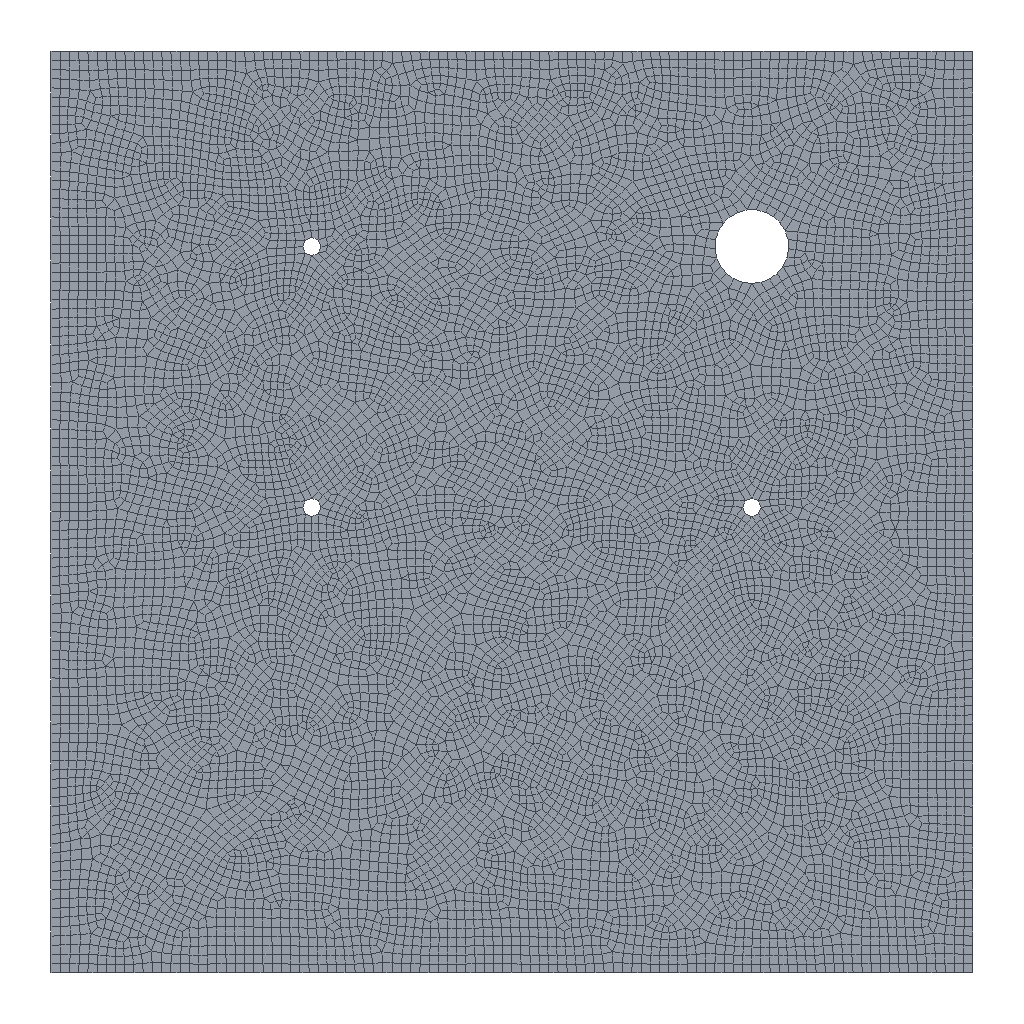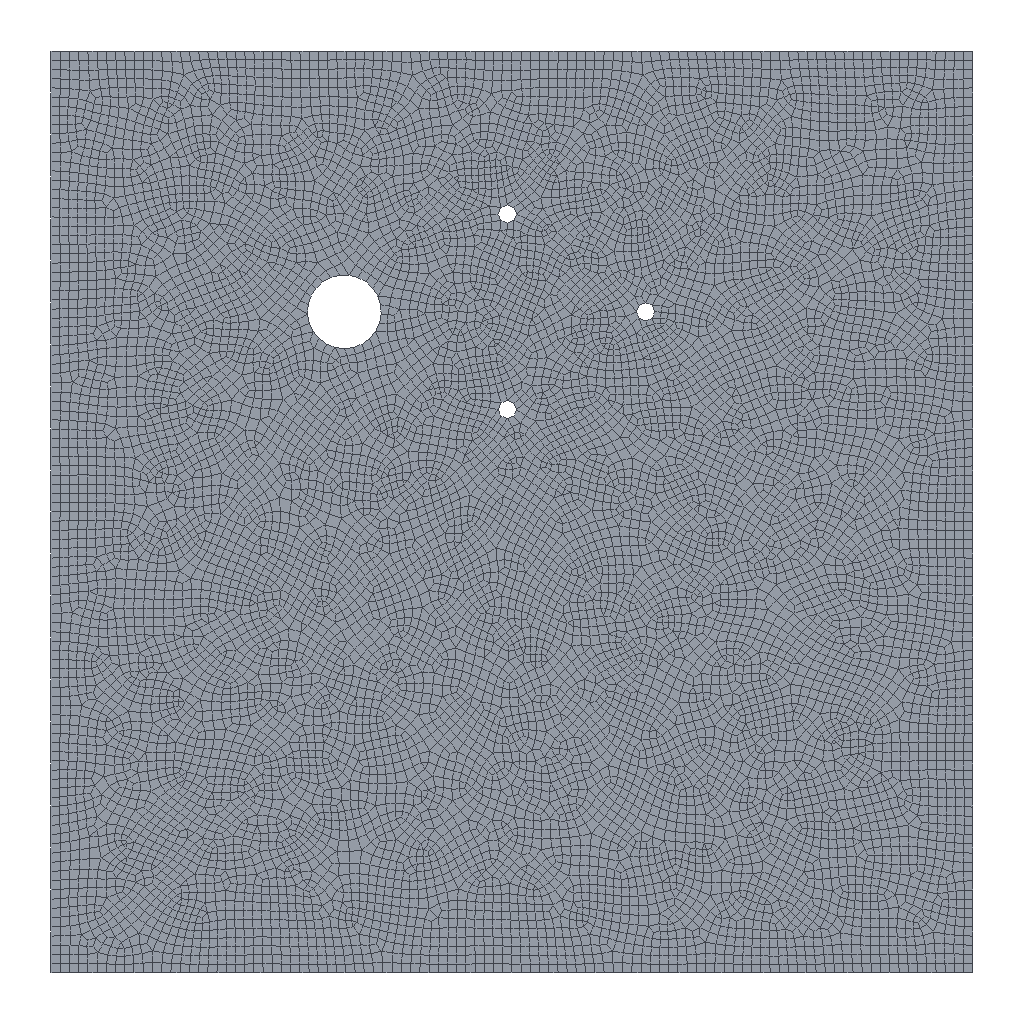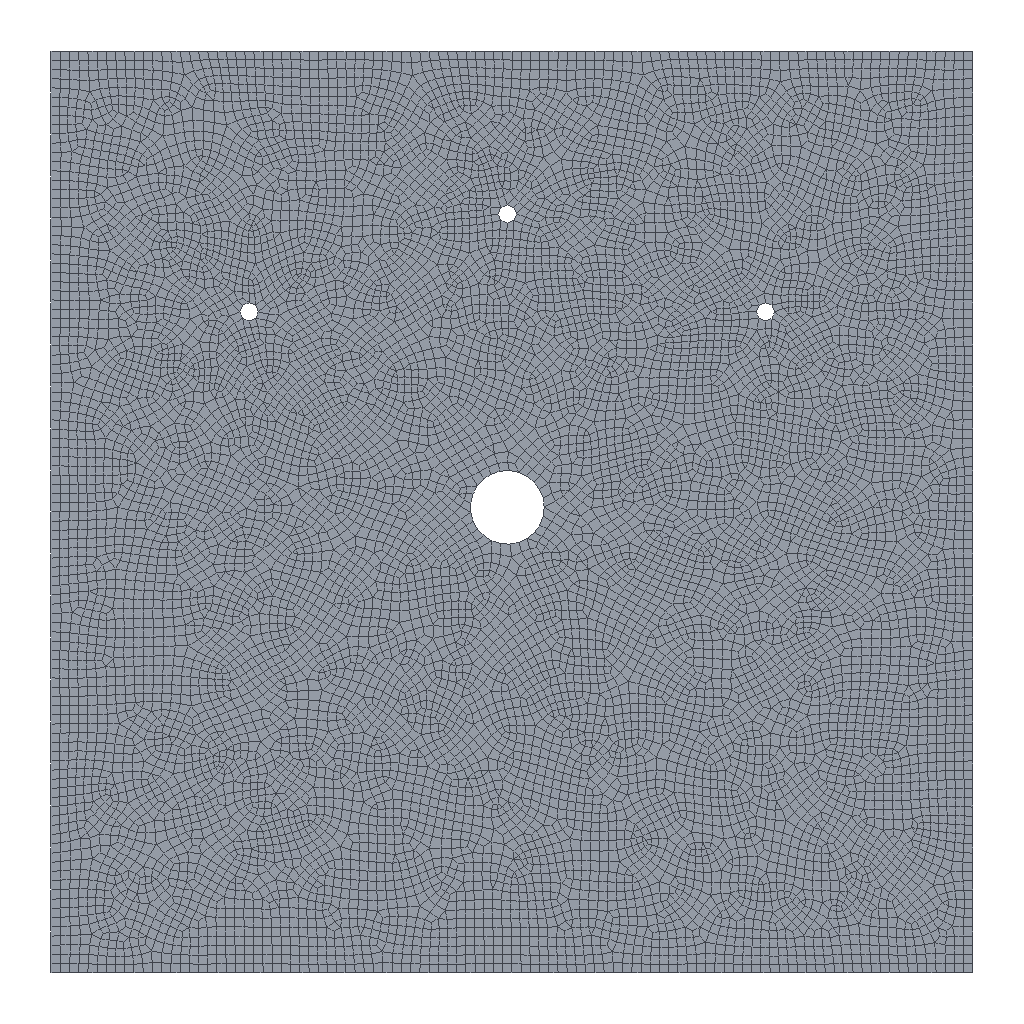Simulation study | abaqus
Set-up summary:
category,name,step,type,value,unit,region
solver,abaqus
solver,version,,,Abaqus/Standard 2020
solver,version,,,Abaqus/Standard 2020
solver,version,,,Abaqus/Standard 2020
units,not stated in the deck,,not stated
analysis,deck1,,static,static
load_step,Step-1,Step-1,static,nlgeom=True
contact,interactions,,,general=0 pairs=0 ties=0
load_step,requested,,,1
mesh,nodes,,,12451
mesh,elements,,,12432
element_type,CPS3,,plane,405
element_type,CPS4R,,plane,12027
load,load commands in deck,,count,3
bc,support commands in deck,,count,1
analysis,deck2,,static,static
load_step,Step-1,Step-1,static,nlgeom=True
contact,interactions,,,general=0 pairs=0 ties=0
load_step,requested,,,1
mesh,nodes,,,12400
mesh,elements,,,12355
element_type,CPS3,,plane,353
element_type,CPS4R,,plane,12002
load,load commands in deck,,count,3
bc,support commands in deck,,count,1
analysis,deck3,,static,static
load_step,Step-1,Step-1,static,nlgeom=True
contact,interactions,,,general=0 pairs=0 ties=0
load_step,requested,,,1
mesh,nodes,,,12295
mesh,elements,,,12253
element_type,CPS3,,plane,359
element_type,CPS4R,,plane,11894
load,load commands in deck,,count,3
bc,support commands in deck,,count,1
material,MATERIAL-1,,in results
material,MATERIAL-1,,in results
material,MATERIAL-1,,in results
check,setup vs results,,match,"per instance, exact: element labels, types and connectivity; labels of the nodes the elements use; coordinates of those nodes at SINGLE_PRECISION in 1 of 1 instance(s)"
check,setup vs results,,match,"per instance, exact: element labels, types and connectivity; labels of the nodes the elements use; coordinates of those nodes at SINGLE_PRECISION in 1 of 1 instance(s)"
check,setup vs results,,match,"per instance, exact: element labels, types and connectivity; labels of the nodes the elements use; coordinates of those nodes at SINGLE_PRECISION in 1 of 1 instance(s)"
Results summary:
result,step,,completed,increments=11 time=1.0/1.0
result,analysis,,,static
result,last_loadstep,,,1
result,analysis steps,,count,1
result,primary field,,,U
result,reaction total,,FX,-0.02379,model units
result,reaction total,,FY,99365.551,model units
result,reaction total,,FZ,0.0,model units
result,step,,completed,increments=11 time=1.0/1.0
result,analysis,,,static
result,last_loadstep,,,1
result,analysis steps,,count,1
result,primary field,,,U
result,reaction total,,FX,-0.3821,model units
result,reaction total,,FY,99365.758,model units
result,reaction total,,FZ,0.0,model units
result,step,,completed,increments=11 time=1.0/1.0
result,analysis,,,static
result,last_loadstep,,,1
result,analysis steps,,count,1
result,primary field,,,U
result,reaction total,,FX,0.4781,model units
result,reaction total,,FY,99365.765,model units
result,reaction total,,FZ,0.0,model units